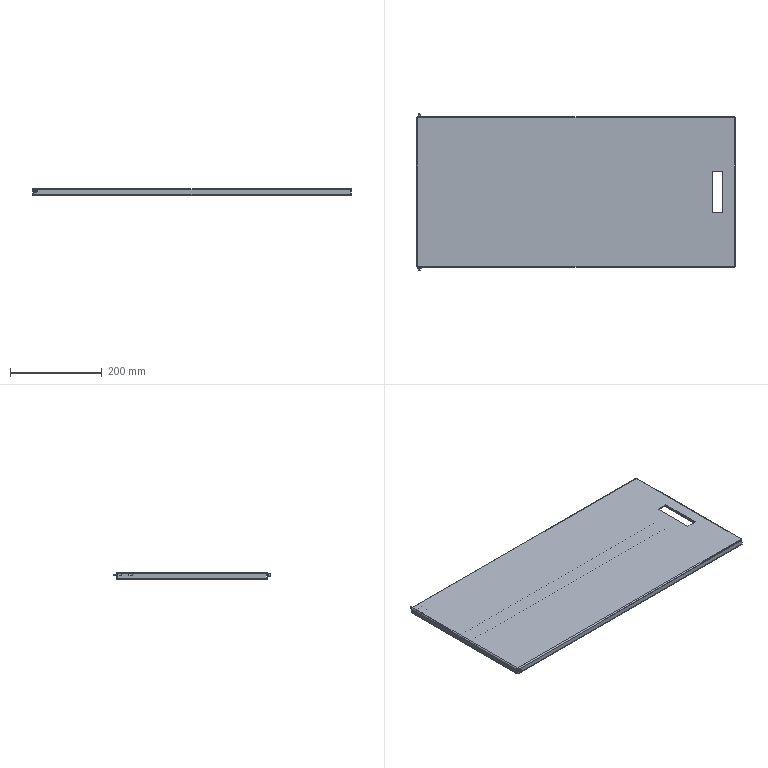Part | SolidWorks | features EdgeFlange 3, FlatPattern 2, ICE 2, MoveCopyBody 2, SMBaseFlange 2, SheetMetal 2, Chamfer 1, Cut 1, HoleWzd 1, Stock 1 | 5 solids | 153 faces | box 693 x 342.263 x 15 mm | volume 608896 mm3 | plane 81 | cylinder 46 | spline 16 | torus 6 | cone 4 | commonest cylinder face diameters 4 x12 1.473 x10 5.473 x8 5 x4 7 x4 3 x2